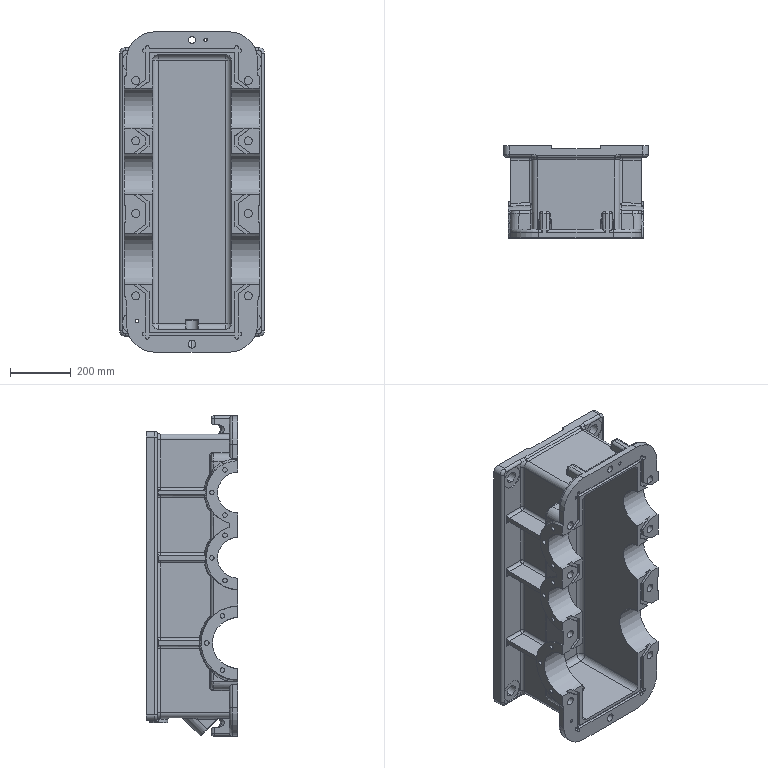Part | SolidWorks | features ICE 51, Fillet 41, MirrorPattern 15, Revolution 5, RevCut 4, Sculpt 3, BlendCut 1, Extrusion 1, Scale 1, SweepCut 1 | 1 solid | 677 faces | box 478.125 x 303.75 x 1058 mm | volume 34791159 mm3 | cylinder 273 | plane 234 | spline 79 | torus 42 | sphere 40 | cone 9 | commonest cylinder face diameters 18.75 x98 15 x36 37.5 x27 26.25 x18 45 x16 7.5 x13